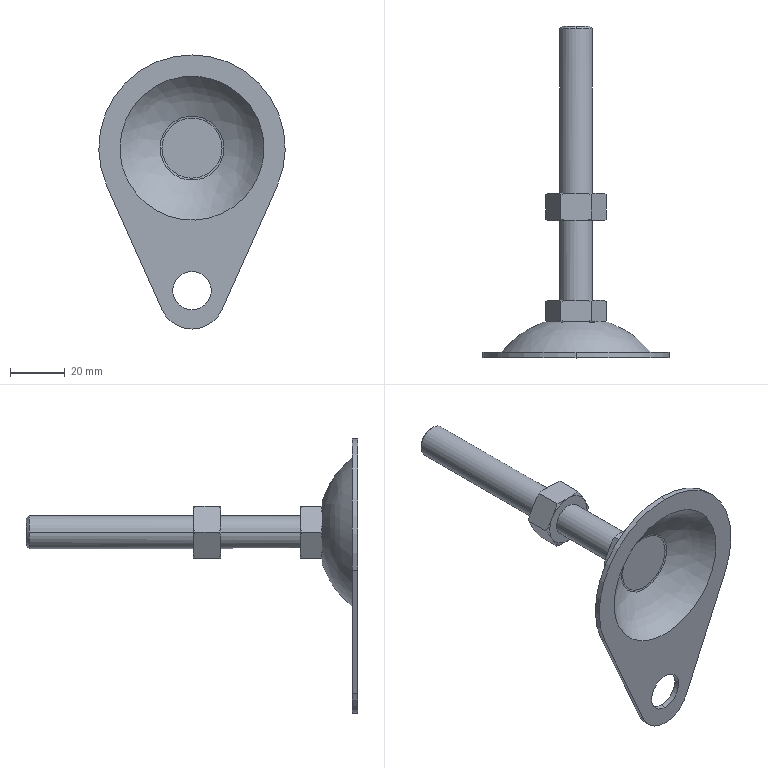Part | SolidWorks | features BaseBody 2 | 2 solids | 65 faces | box 68 x 121 x 100 mm | volume 26277 mm3 | spline 28 | plane 22 | cylinder 9 | cone 6 | commonest cylinder face diameters 10.106 x2 12 x2 14 x2 68 x2 24 x1